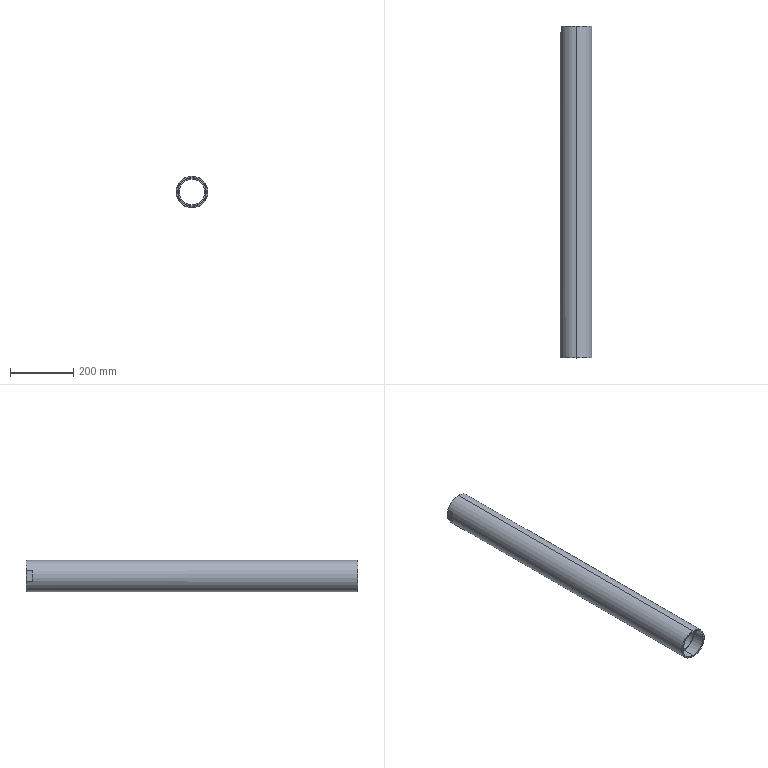Part | SolidWorks | features ICE 4, Chamfer 1, Extrusion 1 | 1 solid | 21 faces | box 100 x 1049 x 100 mm | volume 2893006 mm3 | cylinder 10 | plane 7 | cone 4 | commonest cylinder face diameters 80 x2 81.75 x2 88.75 x2 90 x2 100 x2
STEP:
#1=CARTESIAN_POINT('',(0.,997.,-40.875));
#2=VERTEX_POINT('',#1);
#3=CARTESIAN_POINT('',(0.,997.,40.875));
#4=VERTEX_POINT('',#3);
#5=CARTESIAN_POINT('',(0.,997.,0.));
#6=DIRECTION('',(0.,1.,0.));
#7=DIRECTION('',(0.,0.,1.));
#8=AXIS2_PLACEMENT_3D('',#5,#6,#7);
#9=CIRCLE('',#8,40.875);
#10=EDGE_CURVE('',#2,#4,#9,.T.);
#11=ORIENTED_EDGE('',*,*,#10,.F.);
#12=CARTESIAN_POINT('',(0.,1037.,-40.875));
#13=VERTEX_POINT('',#12);
#14=CARTESIAN_POINT('',(0.,997.,-40.875));
#15=DIRECTION('',(0.,1.,0.));
#16=VECTOR('',#15,1000.);
#17=LINE('',#14,#16);
#18=EDGE_CURVE('',#2,#13,#17,.T.);
#19=ORIENTED_EDGE('',*,*,#18,.T.);
#20=CARTESIAN_POINT('',(0.,1037.,40.875));
#21=VERTEX_POINT('',#20);
#22=CARTESIAN_POINT('',(0.,1037.,0.));
#23=DIRECTION('',(0.,1.,0.));
#24=DIRECTION('',(0.,0.,1.));
#25=AXIS2_PLACEMENT_3D('',#22,#23,#24);
#26=CIRCLE('',#25,40.875);
#27=EDGE_CURVE('',#13,#21,#26,.T.);
#28=ORIENTED_EDGE('',*,*,#27,.T.);
#29=CARTESIAN_POINT('',(0.,997.,40.875));
#30=DIRECTION('',(0.,1.,0.));
#31=VECTOR('',#30,1000.);
#32=LINE('',#29,#31);
#33=EDGE_CURVE('',#4,#21,#32,.T.);
#34=ORIENTED_EDGE('',*,*,#33,.F.);
#35=EDGE_LOOP('',(#11,#19,#28,#34));
#36=FACE_OUTER_BOUND('',#35,.T.);
#37=CARTESIAN_POINT('',(0.,997.,0.));
#38=DIRECTION('',(0.,1.,0.));
#39=DIRECTION('',(0.,0.,1.));
#40=AXIS2_PLACEMENT_3D('',#37,#38,#39);
#41=CYLINDRICAL_SURFACE('',#40,40.875);
#42=ADVANCED_FACE('',(#36),#41,.F.);
#43=CARTESIAN_POINT('',(0.,1.,44.375));
#44=VERTEX_POINT('',#43);
#45=CARTESIAN_POINT('',(0.,1.,-44.375));
#46=VERTEX_POINT('',#45);
#47=CARTESIAN_POINT('',(0.,1.,0.));
#48=DIRECTION('',(0.,-1.,0.));
#49=DIRECTION('',(0.,0.,1.));
#50=AXIS2_PLACEMENT_3D('',#47,#48,#49);
#51=CIRCLE('',#50,44.375);
#52=EDGE_CURVE('',#44,#46,#51,.T.);
#53=ORIENTED_EDGE('',*,*,#52,.F.);
#54=CARTESIAN_POINT('',(0.,0.,45.375));
#55=VERTEX_POINT('',#54);
#56=CARTESIAN_POINT('',(0.,1.,44.375));
#57=DIRECTION('',(0.,-0.7071,0.7071));
#58=VECTOR('',#57,1000.);
#59=LINE('',#56,#58);
#60=EDGE_CURVE('',#44,#55,#59,.T.);
#61=ORIENTED_EDGE('',*,*,#60,.T.);
#62=CARTESIAN_POINT('',(0.,0.,-45.375));
#63=VERTEX_POINT('',#62);
#64=CARTESIAN_POINT('',(0.,0.,0.));
#65=DIRECTION('',(0.,1.,0.));
#66=DIRECTION('',(0.,0.,1.));
#67=AXIS2_PLACEMENT_3D('',#64,#65,#66);
#68=CIRCLE('',#67,45.375);
#69=EDGE_CURVE('',#63,#55,#68,.T.);
#70=ORIENTED_EDGE('',*,*,#69,.F.);
#71=CARTESIAN_POINT('',(0.,1.,-44.375));
#72=DIRECTION('',(0.,-0.7071,-0.7071));
#73=VECTOR('',#72,1000.);
#74=LINE('',#71,#73);
#75=EDGE_CURVE('',#46,#63,#74,.T.);
#76=ORIENTED_EDGE('',*,*,#75,.F.);
#77=EDGE_LOOP('',(#53,#61,#70,#76));
#78=FACE_OUTER_BOUND('',#77,.T.);
#79=CARTESIAN_POINT('',(0.,1.,0.));
#80=DIRECTION('',(0.,-1.,0.));
#81=DIRECTION('',(0.,0.,-1.));
#82=AXIS2_PLACEMENT_3D('',#79,#80,#81);
#83=CONICAL_SURFACE('',#82,44.375,0.7854);
#84=ADVANCED_FACE('',(#78),#83,.F.);
#85=CARTESIAN_POINT('',(0.,0.,-49.));
#86=VERTEX_POINT('',#85);
#87=CARTESIAN_POINT('',(0.,0.,49.));
#88=VERTEX_POINT('',#87);
#89=CARTESIAN_POINT('',(0.,0.,0.));
#90=DIRECTION('',(0.,-1.,0.));
#91=DIRECTION('',(0.,0.,1.));
#92=AXIS2_PLACEMENT_3D('',#89,#90,#91);
#93=CIRCLE('',#92,49.);
#94=EDGE_CURVE('',#86,#88,#93,.T.);
#95=ORIENTED_EDGE('',*,*,#94,.F.);
#96=CARTESIAN_POINT('',(0.,1.,-50.));
#97=VERTEX_POINT('',#96);
#98=CARTESIAN_POINT('',(0.,1.,-50.));
#99=DIRECTION('',(0.,0.7071,-0.7071));
#100=VECTOR('',#99,1000.);
#101=LINE('',#98,#100);
#102=EDGE_CURVE('',#86,#97,#101,.T.);
#103=ORIENTED_EDGE('',*,*,#102,.T.);
#104=CARTESIAN_POINT('',(0.,1.,50.));
#105=VERTEX_POINT('',#104);
#106=CARTESIAN_POINT('',(0.,1.,0.));
#107=DIRECTION('',(0.,1.,0.));
#108=DIRECTION('',(0.,0.,1.));
#109=AXIS2_PLACEMENT_3D('',#106,#107,#108);
#110=CIRCLE('',#109,50.);
#111=EDGE_CURVE('',#105,#97,#110,.T.);
#112=ORIENTED_EDGE('',*,*,#111,.F.);
#113=CARTESIAN_POINT('',(0.,1.,50.));
#114=DIRECTION('',(0.,0.7071,0.7071));
#115=VECTOR('',#114,1000.);
#116=LINE('',#113,#115);
#117=EDGE_CURVE('',#88,#105,#116,.T.);
#118=ORIENTED_EDGE('',*,*,#117,.F.);
#119=EDGE_LOOP('',(#95,#103,#112,#118));
#120=FACE_OUTER_BOUND('',#119,.T.);
#121=CARTESIAN_POINT('',(0.,1.,0.));
#122=DIRECTION('',(0.,1.,0.));
#123=DIRECTION('',(0.,0.,1.));
#124=AXIS2_PLACEMENT_3D('',#121,#122,#123);
#125=CONICAL_SURFACE('',#124,50.,0.7854);
#126=ADVANCED_FACE('',(#120),#125,.T.);
#127=CARTESIAN_POINT('',(0.,40.,44.375));
#128=VERTEX_POINT('',#127);
#129=CARTESIAN_POINT('',(0.,40.,-44.375));
#130=VERTEX_POINT('',#129);
#131=CARTESIAN_POINT('',(0.,40.,0.));
#132=DIRECTION('',(0.,-1.,0.));
#133=DIRECTION('',(0.,0.,-1.));
#134=AXIS2_PLACEMENT_3D('',#131,#132,#133);
#135=CIRCLE('',#134,44.375);
#136=EDGE_CURVE('',#128,#130,#135,.T.);
#137=ORIENTED_EDGE('',*,*,#136,.F.);
#138=CARTESIAN_POINT('',(0.,40.,44.375));
#139=DIRECTION('',(0.,-1.,0.));
#140=VECTOR('',#139,1000.);
#141=LINE('',#138,#140);
#142=EDGE_CURVE('',#128,#44,#141,.T.);
#143=ORIENTED_EDGE('',*,*,#142,.T.);
#144=ORIENTED_EDGE('',*,*,#52,.T.);
#145=CARTESIAN_POINT('',(0.,40.,-44.375));
#146=DIRECTION('',(0.,-1.,0.));
#147=VECTOR('',#146,1000.);
#148=LINE('',#145,#147);
#149=EDGE_CURVE('',#130,#46,#148,.T.);
#150=ORIENTED_EDGE('',*,*,#149,.F.);
#151=EDGE_LOOP('',(#137,#143,#144,#150));
#152=FACE_OUTER_BOUND('',#151,.T.);
#153=CARTESIAN_POINT('',(0.,40.,0.));
#154=DIRECTION('',(0.,-1.,0.));
#155=DIRECTION('',(0.,0.,-1.));
#156=AXIS2_PLACEMENT_3D('',#153,#154,#155);
#157=CYLINDRICAL_SURFACE('',#156,44.375);
#158=ADVANCED_FACE('',(#152),#157,.F.);
#159=CARTESIAN_POINT('',(0.,1037.,-45.));
#160=VERTEX_POINT('',#159);
#161=CARTESIAN_POINT('',(0.,1037.,45.));
#162=VERTEX_POINT('',#161);
#163=CARTESIAN_POINT('',(0.,1037.,0.));
#164=DIRECTION('',(0.,1.,0.));
#165=DIRECTION('',(0.,0.,1.));
#166=AXIS2_PLACEMENT_3D('',#163,#164,#165);
#167=CIRCLE('',#166,45.);
#168=EDGE_CURVE('',#160,#162,#167,.T.);
#169=ORIENTED_EDGE('',*,*,#168,.F.);
#170=CARTESIAN_POINT('',(0.,1049.,-45.));
#171=VERTEX_POINT('',#170);
#172=CARTESIAN_POINT('',(0.,1037.,-45.));
#173=DIRECTION('',(0.,1.,0.));
#174=VECTOR('',#173,1000.);
#175=LINE('',#172,#174);
#176=EDGE_CURVE('',#160,#171,#175,.T.);
#177=ORIENTED_EDGE('',*,*,#176,.T.);
#178=CARTESIAN_POINT('',(0.,1049.,45.));
#179=VERTEX_POINT('',#178);
#180=CARTESIAN_POINT('',(0.,1049.,0.));
#181=DIRECTION('',(0.,1.,0.));
#182=DIRECTION('',(0.,0.,1.));
#183=AXIS2_PLACEMENT_3D('',#180,#181,#182);
#184=CIRCLE('',#183,45.);
#185=EDGE_CURVE('',#171,#179,#184,.T.);
#186=ORIENTED_EDGE('',*,*,#185,.T.);
#187=CARTESIAN_POINT('',(0.,1037.,45.));
#188=DIRECTION('',(0.,1.,0.));
#189=VECTOR('',#188,1000.);
#190=LINE('',#187,#189);
#191=EDGE_CURVE('',#162,#179,#190,.T.);
#192=ORIENTED_EDGE('',*,*,#191,.F.);
#193=EDGE_LOOP('',(#169,#177,#186,#192));
#194=FACE_OUTER_BOUND('',#193,.T.);
#195=CARTESIAN_POINT('',(0.,1037.,0.));
#196=DIRECTION('',(0.,1.,0.));
#197=DIRECTION('',(0.,0.,1.));
#198=AXIS2_PLACEMENT_3D('',#195,#196,#197);
#199=CYLINDRICAL_SURFACE('',#198,45.);
#200=ADVANCED_FACE('',(#194),#199,.F.);
#201=CARTESIAN_POINT('',(0.,1049.,50.));
#202=VERTEX_POINT('',#201);
#203=CARTESIAN_POINT('',(0.,1049.,-50.));
#204=VERTEX_POINT('',#203);
#205=CARTESIAN_POINT('',(0.,1049.,0.));
#206=DIRECTION('',(0.,1.,0.));
#207=DIRECTION('',(0.,0.,1.));
#208=AXIS2_PLACEMENT_3D('',#205,#206,#207);
#209=CIRCLE('',#208,50.);
#210=EDGE_CURVE('',#202,#204,#209,.T.);
#211=ORIENTED_EDGE('',*,*,#210,.F.);
#212=CARTESIAN_POINT('',(0.,1049.,50.));
#213=DIRECTION('',(0.,-1.,0.));
#214=VECTOR('',#213,1000.);
#215=LINE('',#212,#214);
#216=EDGE_CURVE('',#202,#105,#215,.T.);
#217=ORIENTED_EDGE('',*,*,#216,.T.);
#218=ORIENTED_EDGE('',*,*,#111,.T.);
#219=CARTESIAN_POINT('',(0.,1049.,-50.));
#220=DIRECTION('',(0.,-1.,0.));
#221=VECTOR('',#220,1000.);
#222=LINE('',#219,#221);
#223=EDGE_CURVE('',#204,#97,#222,.T.);
#224=ORIENTED_EDGE('',*,*,#223,.F.);
#225=EDGE_LOOP('',(#211,#217,#218,#224));
#226=FACE_OUTER_BOUND('',#225,.T.);
#227=CARTESIAN_POINT('',(0.,1049.,0.));
#228=DIRECTION('',(0.,-1.,0.));
#229=DIRECTION('',(0.,0.,-1.));
#230=AXIS2_PLACEMENT_3D('',#227,#228,#229);
#231=CYLINDRICAL_SURFACE('',#230,50.);
#232=ADVANCED_FACE('',(#226),#231,.T.);
#233=CARTESIAN_POINT('',(0.,997.,-40.));
#234=VERTEX_POINT('',#233);
#235=CARTESIAN_POINT('',(0.,997.,40.));
#236=VERTEX_POINT('',#235);
#237=CARTESIAN_POINT('',(0.,997.,0.));
#238=DIRECTION('',(0.,1.,0.));
#239=DIRECTION('',(0.,0.,1.));
#240=AXIS2_PLACEMENT_3D('',#237,#238,#239);
#241=CIRCLE('',#240,40.);
#242=EDGE_CURVE('',#234,#236,#241,.T.);
#243=ORIENTED_EDGE('',*,*,#242,.T.);
#244=CARTESIAN_POINT('',(0.,40.,40.));
#245=VERTEX_POINT('',#244);
#246=CARTESIAN_POINT('',(0.,1049.,40.));
#247=DIRECTION('',(0.,-1.,0.));
#248=VECTOR('',#247,1000.);
#249=LINE('',#246,#248);
#250=EDGE_CURVE('',#236,#245,#249,.T.);
#251=ORIENTED_EDGE('',*,*,#250,.T.);
#252=CARTESIAN_POINT('',(0.,40.,-40.));
#253=VERTEX_POINT('',#252);
#254=CARTESIAN_POINT('',(0.,40.,0.));
#255=DIRECTION('',(0.,-1.,0.));
#256=DIRECTION('',(0.,0.,-1.));
#257=AXIS2_PLACEMENT_3D('',#254,#255,#256);
#258=CIRCLE('',#257,40.);
#259=EDGE_CURVE('',#245,#253,#258,.T.);
#260=ORIENTED_EDGE('',*,*,#259,.T.);
#261=CARTESIAN_POINT('',(0.,1049.,-40.));
#262=DIRECTION('',(0.,-1.,0.));
#263=VECTOR('',#262,1000.);
#264=LINE('',#261,#263);
#265=EDGE_CURVE('',#234,#253,#264,.T.);
#266=ORIENTED_EDGE('',*,*,#265,.F.);
#267=EDGE_LOOP('',(#243,#251,#260,#266));
#268=FACE_OUTER_BOUND('',#267,.T.);
#269=CARTESIAN_POINT('',(0.,1049.,0.));
#270=DIRECTION('',(0.,-1.,0.));
#271=DIRECTION('',(0.,0.,-1.));
#272=AXIS2_PLACEMENT_3D('',#269,#270,#271);
#273=CYLINDRICAL_SURFACE('',#272,40.);
#274=ADVANCED_FACE('',(#268),#273,.F.);
#275=ORIENTED_EDGE('',*,*,#250,.F.);
#276=CARTESIAN_POINT('',(0.,997.,0.));
#277=DIRECTION('',(0.,1.,0.));
#278=DIRECTION('',(0.,0.,1.));
#279=AXIS2_PLACEMENT_3D('',#276,#277,#278);
#280=CIRCLE('',#279,40.);
#281=EDGE_CURVE('',#236,#234,#280,.T.);
#282=ORIENTED_EDGE('',*,*,#281,.T.);
#283=ORIENTED_EDGE('',*,*,#265,.T.);
#284=CARTESIAN_POINT('',(0.,40.,0.));
#285=DIRECTION('',(0.,-1.,0.));
#286=DIRECTION('',(0.,0.,-1.));
#287=AXIS2_PLACEMENT_3D('',#284,#285,#286);
#288=CIRCLE('',#287,40.);
#289=EDGE_CURVE('',#253,#245,#288,.T.);
#290=ORIENTED_EDGE('',*,*,#289,.T.);
#291=EDGE_LOOP('',(#275,#282,#283,#290));
#292=FACE_OUTER_BOUND('',#291,.T.);
#293=CARTESIAN_POINT('',(0.,1049.,0.));
#294=DIRECTION('',(0.,-1.,0.));
#295=DIRECTION('',(0.,0.,-1.));
#296=AXIS2_PLACEMENT_3D('',#293,#294,#295);
#297=CYLINDRICAL_SURFACE('',#296,40.);
#298=ADVANCED_FACE('',(#292),#297,.F.);
#299=CARTESIAN_POINT('',(-47.,1049.,17.059));
#300=VERTEX_POINT('',#299);
#301=CARTESIAN_POINT('',(-47.,1049.,-17.059));
#302=VERTEX_POINT('',#301);
#303=CARTESIAN_POINT('',(-47.,1049.,0.));
#304=DIRECTION('',(0.,0.,-1.));
#305=VECTOR('',#304,1000.);
#306=LINE('',#303,#305);
#307=EDGE_CURVE('',#300,#302,#306,.T.);
#308=ORIENTED_EDGE('',*,*,#307,.F.);
#309=CARTESIAN_POINT('',(0.,1049.,0.));
#310=DIRECTION('',(0.,1.,0.));
#311=DIRECTION('',(0.,0.,1.));
#312=AXIS2_PLACEMENT_3D('',#309,#310,#311);
#313=CIRCLE('',#312,50.);
#314=EDGE_CURVE('',#300,#202,#313,.T.);
#315=ORIENTED_EDGE('',*,*,#314,.T.);
#316=ORIENTED_EDGE('',*,*,#210,.T.);
#317=CARTESIAN_POINT('',(0.,1049.,0.));
#318=DIRECTION('',(0.,1.,0.));
#319=DIRECTION('',(0.,0.,1.));
#320=AXIS2_PLACEMENT_3D('',#317,#318,#319);
#321=CIRCLE('',#320,50.);
#322=EDGE_CURVE('',#204,#302,#321,.T.);
#323=ORIENTED_EDGE('',*,*,#322,.T.);
#324=EDGE_LOOP('',(#308,#315,#316,#323));
#325=FACE_OUTER_BOUND('',#324,.T.);
#326=CARTESIAN_POINT('',(0.,1049.,0.));
#327=DIRECTION('',(0.,1.,0.));
#328=DIRECTION('',(0.,0.,1.));
#329=AXIS2_PLACEMENT_3D('',#326,#327,#328);
#330=CIRCLE('',#329,45.);
#331=EDGE_CURVE('',#179,#171,#330,.T.);
#332=ORIENTED_EDGE('',*,*,#331,.F.);
#333=ORIENTED_EDGE('',*,*,#185,.F.);
#334=EDGE_LOOP('',(#332,#333));
#335=FACE_BOUND('',#334,.T.);
#336=CARTESIAN_POINT('',(0.,1049.,0.));
#337=DIRECTION('',(0.,1.,0.));
#338=DIRECTION('',(0.,0.,1.));
#339=AXIS2_PLACEMENT_3D('',#336,#337,#338);
#340=PLANE('',#339);
#341=ADVANCED_FACE('',(#325,#335),#340,.T.);
#342=CARTESIAN_POINT('',(0.,0.,0.));
#343=DIRECTION('',(0.,-1.,0.));
#344=DIRECTION('',(0.,0.,1.));
#345=AXIS2_PLACEMENT_3D('',#342,#343,#344);
#346=CIRCLE('',#345,49.);
#347=EDGE_CURVE('',#88,#86,#346,.T.);
#348=ORIENTED_EDGE('',*,*,#347,.T.);
#349=ORIENTED_EDGE('',*,*,#94,.T.);
#350=EDGE_LOOP('',(#348,#349));
#351=FACE_OUTER_BOUND('',#350,.T.);
#352=ORIENTED_EDGE('',*,*,#69,.T.);
#353=CARTESIAN_POINT('',(0.,0.,0.));
#354=DIRECTION('',(0.,1.,0.));
#355=DIRECTION('',(0.,0.,1.));
#356=AXIS2_PLACEMENT_3D('',#353,#354,#355);
#357=CIRCLE('',#356,45.375);
#358=EDGE_CURVE('',#55,#63,#357,.T.);
#359=ORIENTED_EDGE('',*,*,#358,.T.);
#360=EDGE_LOOP('',(#352,#359));
#361=FACE_BOUND('',#360,.T.);
#362=CARTESIAN_POINT('',(0.,0.,0.));
#363=DIRECTION('',(0.,1.,0.));
#364=DIRECTION('',(0.,0.,1.));
#365=AXIS2_PLACEMENT_3D('',#362,#363,#364);
#366=PLANE('',#365);
#367=ADVANCED_FACE('',(#351,#361),#366,.F.);
#368=ORIENTED_EDGE('',*,*,#216,.F.);
#369=ORIENTED_EDGE('',*,*,#314,.F.);
#370=CARTESIAN_POINT('',(-47.,1029.,17.059));
#371=VERTEX_POINT('',#370);
#372=CARTESIAN_POINT('',(-47.,1049.,17.059));
#373=DIRECTION('',(0.,-1.,0.));
#374=VECTOR('',#373,1000.);
#375=LINE('',#372,#374);
#376=EDGE_CURVE('',#300,#371,#375,.T.);
#377=ORIENTED_EDGE('',*,*,#376,.T.);
#378=CARTESIAN_POINT('',(-47.,1029.,-17.059));
#379=VERTEX_POINT('',#378);
#380=CARTESIAN_POINT('',(0.,1029.,0.));
#381=DIRECTION('',(0.,-1.,0.));
#382=DIRECTION('',(0.,0.,-1.));
#383=AXIS2_PLACEMENT_3D('',#380,#381,#382);
#384=CIRCLE('',#383,50.);
#385=EDGE_CURVE('',#371,#379,#384,.T.);
#386=ORIENTED_EDGE('',*,*,#385,.T.);
#387=CARTESIAN_POINT('',(-47.,1049.,-17.059));
#388=DIRECTION('',(0.,1.,0.));
#389=VECTOR('',#388,1000.);
#390=LINE('',#387,#389);
#391=EDGE_CURVE('',#379,#302,#390,.T.);
#392=ORIENTED_EDGE('',*,*,#391,.T.);
#393=ORIENTED_EDGE('',*,*,#322,.F.);
#394=ORIENTED_EDGE('',*,*,#223,.T.);
#395=CARTESIAN_POINT('',(0.,1.,0.));
#396=DIRECTION('',(0.,1.,0.));
#397=DIRECTION('',(0.,0.,1.));
#398=AXIS2_PLACEMENT_3D('',#395,#396,#397);
#399=CIRCLE('',#398,50.);
#400=EDGE_CURVE('',#97,#105,#399,.T.);
#401=ORIENTED_EDGE('',*,*,#400,.T.);
#402=EDGE_LOOP('',(#368,#369,#377,#386,#392,#393,#394,#401));
#403=FACE_OUTER_BOUND('',#402,.T.);
#404=CARTESIAN_POINT('',(0.,1049.,0.));
#405=DIRECTION('',(0.,-1.,0.));
#406=DIRECTION('',(0.,0.,-1.));
#407=AXIS2_PLACEMENT_3D('',#404,#405,#406);
#408=CYLINDRICAL_SURFACE('',#407,50.);
#409=ADVANCED_FACE('',(#403),#408,.T.);
#410=ORIENTED_EDGE('',*,*,#176,.F.);
#411=CARTESIAN_POINT('',(0.,1037.,0.));
#412=DIRECTION('',(0.,1.,0.));
#413=DIRECTION('',(0.,0.,1.));
#414=AXIS2_PLACEMENT_3D('',#411,#412,#413);
#415=CIRCLE('',#414,45.);
#416=EDGE_CURVE('',#162,#160,#415,.T.);
#417=ORIENTED_EDGE('',*,*,#416,.F.);
#418=ORIENTED_EDGE('',*,*,#191,.T.);
#419=ORIENTED_EDGE('',*,*,#331,.T.);
#420=EDGE_LOOP('',(#410,#417,#418,#419));
#421=FACE_OUTER_BOUND('',#420,.T.);
#422=CARTESIAN_POINT('',(0.,1037.,0.));
#423=DIRECTION('',(0.,1.,0.));
#424=DIRECTION('',(0.,0.,1.));
#425=AXIS2_PLACEMENT_3D('',#422,#423,#424);
#426=CYLINDRICAL_SURFACE('',#425,45.);
#427=ADVANCED_FACE('',(#421),#426,.F.);
#428=CARTESIAN_POINT('',(0.,1037.,0.));
#429=DIRECTION('',(0.,1.,0.));
#430=DIRECTION('',(0.,0.,1.));
#431=AXIS2_PLACEMENT_3D('',#428,#429,#430);
#432=CIRCLE('',#431,40.875);
#433=EDGE_CURVE('',#21,#13,#432,.T.);
#434=ORIENTED_EDGE('',*,*,#433,.F.);
#435=ORIENTED_EDGE('',*,*,#27,.F.);
#436=EDGE_LOOP('',(#434,#435));
#437=FACE_BOUND('',#436,.T.);
#438=ORIENTED_EDGE('',*,*,#416,.T.);
#439=ORIENTED_EDGE('',*,*,#168,.T.);
#440=EDGE_LOOP('',(#438,#439));
#441=FACE_OUTER_BOUND('',#440,.T.);
#442=CARTESIAN_POINT('',(0.,1037.,0.));
#443=DIRECTION('',(0.,1.,0.));
#444=DIRECTION('',(0.,0.,1.));
#445=AXIS2_PLACEMENT_3D('',#442,#443,#444);
#446=PLANE('',#445);
#447=ADVANCED_FACE('',(#437,#441),#446,.T.);
#448=ORIENTED_EDGE('',*,*,#142,.F.);
#449=CARTESIAN_POINT('',(0.,40.,0.));
#450=DIRECTION('',(0.,-1.,0.));
#451=DIRECTION('',(0.,0.,-1.));
#452=AXIS2_PLACEMENT_3D('',#449,#450,#451);
#453=CIRCLE('',#452,44.375);
#454=EDGE_CURVE('',#130,#128,#453,.T.);
#455=ORIENTED_EDGE('',*,*,#454,.F.);
#456=ORIENTED_EDGE('',*,*,#149,.T.);
#457=CARTESIAN_POINT('',(0.,1.,0.));
#458=DIRECTION('',(0.,-1.,0.));
#459=DIRECTION('',(0.,0.,1.));
#460=AXIS2_PLACEMENT_3D('',#457,#458,#459);
#461=CIRCLE('',#460,44.375);
#462=EDGE_CURVE('',#46,#44,#461,.T.);
#463=ORIENTED_EDGE('',*,*,#462,.T.);
#464=EDGE_LOOP('',(#448,#455,#456,#463));
#465=FACE_OUTER_BOUND('',#464,.T.);
#466=CARTESIAN_POINT('',(0.,40.,0.));
#467=DIRECTION('',(0.,-1.,0.));
#468=DIRECTION('',(0.,0.,-1.));
#469=AXIS2_PLACEMENT_3D('',#466,#467,#468);
#470=CYLINDRICAL_SURFACE('',#469,44.375);
#471=ADVANCED_FACE('',(#465),#470,.F.);
#472=ORIENTED_EDGE('',*,*,#289,.F.);
#473=ORIENTED_EDGE('',*,*,#259,.F.);
#474=EDGE_LOOP('',(#472,#473));
#475=FACE_BOUND('',#474,.T.);
#476=ORIENTED_EDGE('',*,*,#454,.T.);
#477=ORIENTED_EDGE('',*,*,#136,.T.);
#478=EDGE_LOOP('',(#476,#477));
#479=FACE_OUTER_BOUND('',#478,.T.);
#480=CARTESIAN_POINT('',(0.,40.,0.));
#481=DIRECTION('',(0.,-1.,0.));
#482=DIRECTION('',(0.,0.,-1.));
#483=AXIS2_PLACEMENT_3D('',#480,#481,#482);
#484=PLANE('',#483);
#485=ADVANCED_FACE('',(#475,#479),#484,.T.);
#486=ORIENTED_EDGE('',*,*,#102,.F.);
#487=ORIENTED_EDGE('',*,*,#347,.F.);
#488=ORIENTED_EDGE('',*,*,#117,.T.);
#489=ORIENTED_EDGE('',*,*,#400,.F.);
#490=EDGE_LOOP('',(#486,#487,#488,#489));
#491=FACE_OUTER_BOUND('',#490,.T.);
#492=CARTESIAN_POINT('',(0.,1.,0.));
#493=DIRECTION('',(0.,1.,0.));
#494=DIRECTION('',(0.,0.,1.));
#495=AXIS2_PLACEMENT_3D('',#492,#493,#494);
#496=CONICAL_SURFACE('',#495,50.,0.7854);
#497=ADVANCED_FACE('',(#491),#496,.T.);
#498=ORIENTED_EDGE('',*,*,#60,.F.);
#499=ORIENTED_EDGE('',*,*,#462,.F.);
#500=ORIENTED_EDGE('',*,*,#75,.T.);
#501=ORIENTED_EDGE('',*,*,#358,.F.);
#502=EDGE_LOOP('',(#498,#499,#500,#501));
#503=FACE_OUTER_BOUND('',#502,.T.);
#504=CARTESIAN_POINT('',(0.,1.,0.));
#505=DIRECTION('',(0.,-1.,0.));
#506=DIRECTION('',(0.,0.,-1.));
#507=AXIS2_PLACEMENT_3D('',#504,#505,#506);
#508=CONICAL_SURFACE('',#507,44.375,0.7854);
#509=ADVANCED_FACE('',(#503),#508,.F.);
#510=ORIENTED_EDGE('',*,*,#18,.F.);
#511=CARTESIAN_POINT('',(0.,997.,0.));
#512=DIRECTION('',(0.,1.,0.));
#513=DIRECTION('',(0.,0.,1.));
#514=AXIS2_PLACEMENT_3D('',#511,#512,#513);
#515=CIRCLE('',#514,40.875);
#516=EDGE_CURVE('',#4,#2,#515,.T.);
#517=ORIENTED_EDGE('',*,*,#516,.F.);
#518=ORIENTED_EDGE('',*,*,#33,.T.);
#519=ORIENTED_EDGE('',*,*,#433,.T.);
#520=EDGE_LOOP('',(#510,#517,#518,#519));
#521=FACE_OUTER_BOUND('',#520,.T.);
#522=CARTESIAN_POINT('',(0.,997.,0.));
#523=DIRECTION('',(0.,1.,0.));
#524=DIRECTION('',(0.,0.,1.));
#525=AXIS2_PLACEMENT_3D('',#522,#523,#524);
#526=CYLINDRICAL_SURFACE('',#525,40.875);
#527=ADVANCED_FACE('',(#521),#526,.F.);
#528=ORIENTED_EDGE('',*,*,#242,.F.);
#529=ORIENTED_EDGE('',*,*,#281,.F.);
#530=EDGE_LOOP('',(#528,#529));
#531=FACE_BOUND('',#530,.T.);
#532=ORIENTED_EDGE('',*,*,#516,.T.);
#533=ORIENTED_EDGE('',*,*,#10,.T.);
#534=EDGE_LOOP('',(#532,#533));
#535=FACE_OUTER_BOUND('',#534,.T.);
#536=CARTESIAN_POINT('',(0.,997.,0.));
#537=DIRECTION('',(0.,1.,0.));
#538=DIRECTION('',(0.,0.,1.));
#539=AXIS2_PLACEMENT_3D('',#536,#537,#538);
#540=PLANE('',#539);
#541=ADVANCED_FACE('',(#531,#535),#540,.T.);
#542=ORIENTED_EDGE('',*,*,#307,.T.);
#543=ORIENTED_EDGE('',*,*,#391,.F.);
#544=CARTESIAN_POINT('',(-47.,1029.,-50.));
#545=DIRECTION('',(0.,0.,1.));
#546=VECTOR('',#545,1000.);
#547=LINE('',#544,#546);
#548=EDGE_CURVE('',#379,#371,#547,.T.);
#549=ORIENTED_EDGE('',*,*,#548,.T.);
#550=ORIENTED_EDGE('',*,*,#376,.F.);
#551=EDGE_LOOP('',(#542,#543,#549,#550));
#552=FACE_OUTER_BOUND('',#551,.T.);
#553=CARTESIAN_POINT('',(-47.,1069.,-50.));
#554=DIRECTION('',(1.,0.,0.));
#555=DIRECTION('',(0.,0.,-1.));
#556=AXIS2_PLACEMENT_3D('',#553,#554,#555);
#557=PLANE('',#556);
#558=ADVANCED_FACE('',(#552),#557,.F.);
#559=ORIENTED_EDGE('',*,*,#548,.F.);
#560=ORIENTED_EDGE('',*,*,#385,.F.);
#561=EDGE_LOOP('',(#559,#560));
#562=FACE_OUTER_BOUND('',#561,.T.);
#563=CARTESIAN_POINT('',(-53.,1029.,-50.));
#564=DIRECTION('',(0.,-1.,0.));
#565=DIRECTION('',(0.,0.,-1.));
#566=AXIS2_PLACEMENT_3D('',#563,#564,#565);
#567=PLANE('',#566);
#568=ADVANCED_FACE('',(#562),#567,.F.);
#569=CLOSED_SHELL('',(#42,#84,#126,#158,#200,#232,#274,#298,#341,#367,#409,#427,#447,#471,#485,#497,#509,#527,#541,#558,#568));
#570=MANIFOLD_SOLID_BREP('',#569);
#571=CARTESIAN_POINT('',(0.,0.,0.));
#572=DIRECTION('',(0.,0.,1.));
#573=DIRECTION('',(1.,0.,0.));
#574=AXIS2_PLACEMENT_3D('',#571,#572,#573);
#575=(LENGTH_UNIT()NAMED_UNIT(*)SI_UNIT(.MILLI.,.METRE.));
#576=UNCERTAINTY_MEASURE_WITH_UNIT(LENGTH_MEASURE(0.00001),#575,'','');
#577=(NAMED_UNIT(*)PLANE_ANGLE_UNIT()SI_UNIT($,.RADIAN.));
#578=(NAMED_UNIT(*)SI_UNIT($,.STERADIAN.)SOLID_ANGLE_UNIT());
#579=(GEOMETRIC_REPRESENTATION_CONTEXT(3)GLOBAL_UNCERTAINTY_ASSIGNED_CONTEXT((#576))GLOBAL_UNIT_ASSIGNED_CONTEXT((#575,#577,#578))REPRESENTATION_CONTEXT('',''));
#580=ADVANCED_BREP_SHAPE_REPRESENTATION('',(#570,#574),#579);